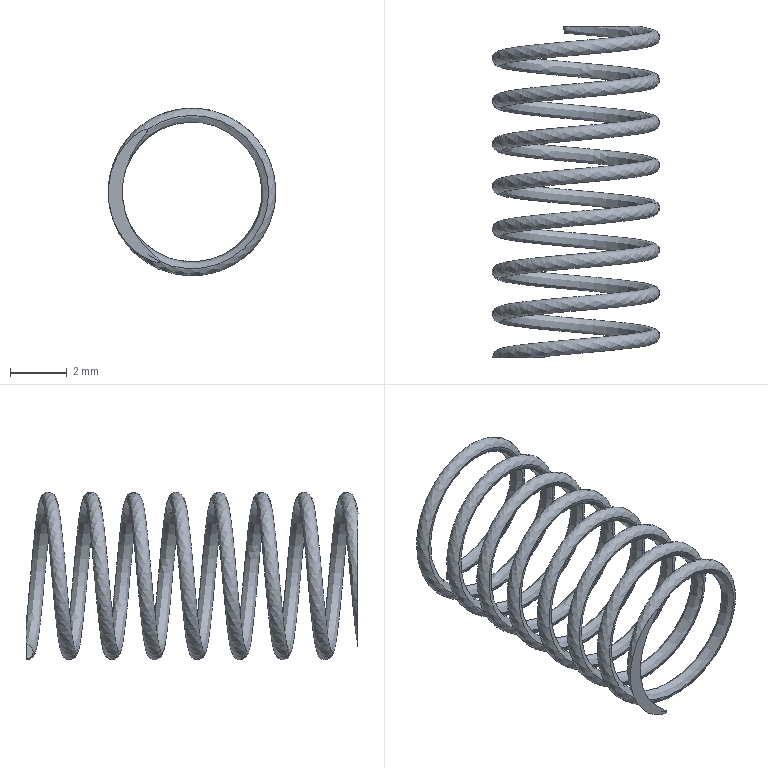Part | SolidWorks | features BaseBody 1 | 1 solid | 5 faces | box 5.9 x 11.685 x 5.904 mm | volume 26.032 mm3 | plane 3 | spline 2